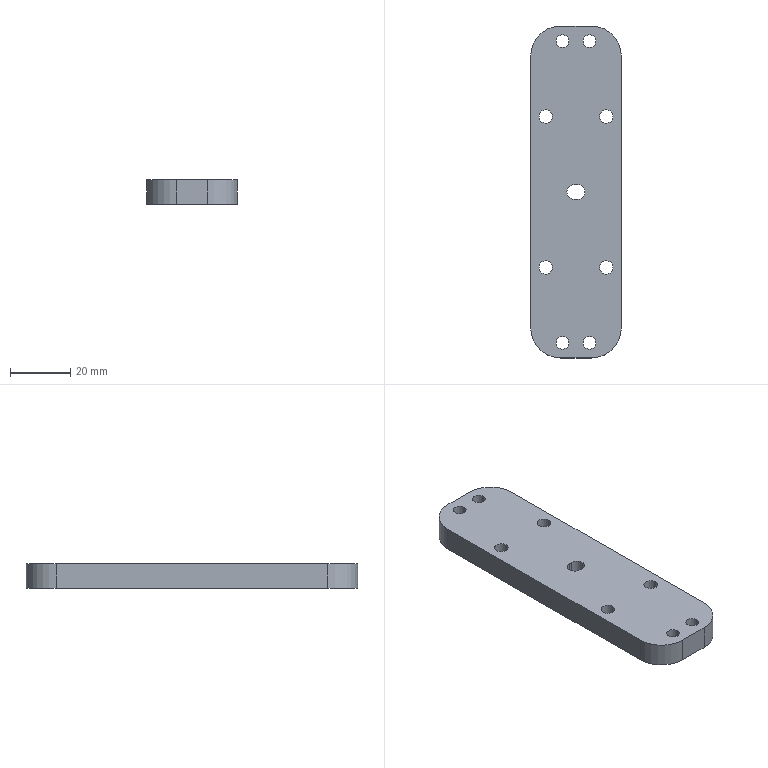Part | STEP file | C02 | 1 solid | 43 faces | box 30 x 110 x 8 mm | volume 23959 mm3 | cylinder 31 | plane 12 | commonest cylinder face diameters 4.2 x8 4.5 x8 8 x8 20 x4 5 x3